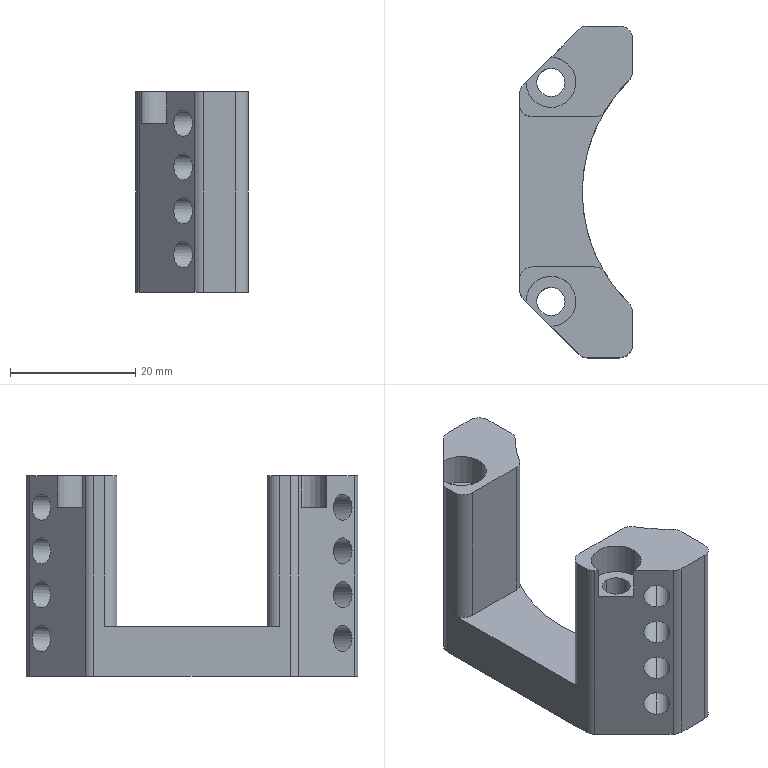CAM job | Mastercam | 3-axis milling, drilling | stock box 25 x 60 x 32 mm
Tools:
tool_number,name,type,diameter_mm,corner_radius_mm,flutes,flute_length_mm,overall_length_mm,shoulder_length_mm,holder_diameter_mm,length_offset,diameter_offset,default_rpm,default_feed_mm_min,default_plunge_mm_min,coolant
4,4 Flat End Mill,end mill,4,0,4,25,75,25,50,4,4,2500,300,600,COOL_OFF
5,4 Chamfer Mill,chamfer mill,4,0,4,25,75,30,50,5,5,6250,750,600,COOL_OFF
11,12 Flat End Mill,end mill,12,0,4,25,75,25,50,11,11,833,99.96,600,COOL_OFF
12,12 Flat End Mill,end mill,12,0,4,25,75,25,50,12,12,833,99.96,600,COOL_OFF
24,100 Flat End Mill,end mill,100,0,4,25,75,25,50,24,24,100,12,600,COOL_OFF
Operations:
seq,operation,operation_type,tool_number,tool_name,tool_diameter_mm,spindle_rpm,feed_mm_min,plunge_mm_min,retract_mm_min,cycle_time_s,wcs,posted,nc_file
1,Facing - [WCS: Plane] - [Tplane: Plane],Facing,24,100 Flat End Mill,100,4000,3000,600,1200,37.654,Plane,yes,.nc
2,3D High Speed (Dynamic OptiRough) - [WCS: Plane] - [Tplane: Plane],HighSpeed3D,11,12 Flat End Mill,12,7000,3000,600,1200,112.101,Plane,yes,.nc
3,Contour (Ramp) - [WCS: Plane] - [Tplane: Plane],Contour,4,4 Flat End Mill,4,6500,2500,600,1200,11.483,Plane,yes,.nc
4,Contour (2D) - [WCS: Plane] - [Tplane: Plane],Contour,4,4 Flat End Mill,4,6500,1000,600,1200,3.961,Plane,yes,.nc
5,2D High Speed (2D Area Mill) - [WCS: Plane] - [Tplane: Plane],HighSpeed2D,12,12 Flat End Mill,12,6000,1000,600,1200,8.271,Plane,yes,.nc
6,Contour (2D) - [WCS: Plane] - [Tplane: Plane],Contour,12,12 Flat End Mill,12,6000,1000,600,1200,29.607,Plane,yes,.nc
7,Contour (2D) - [WCS: Plane] - [Tplane: Plane],Contour,12,12 Flat End Mill,12,6000,1000,600,1200,11.519,Plane,yes,.nc
8,Drill/Counterbore - [WCS: Plane] - [Tplane: Plane],Drill,5,4 Chamfer Mill,4,6000,200,600,1200,1.977,Plane,yes,.nc
9,Contour (2D chamfer) - [WCS: Plane] - [Tplane: Plane],Contour,5,4 Chamfer Mill,4,6000,1000,600,1200,10.077,Plane,yes,.nc
10,2D High Speed (2D Area Mill) - [WCS: Plane-1] - [Tplane: Plane-1],HighSpeed2D,4,4 Flat End Mill,4,7000,3000,600,1200,189.428,Plane-1,yes,.nc
11,Contour (2D) - [WCS: Plane-1] - [Tplane: Plane-1],Contour,4,4 Flat End Mill,4,6000,1000,600,1200,8.694,Plane-1,yes,.nc
12,Contour (2D chamfer) - [WCS: Plane-1] - [Tplane: Plane-1],Contour,5,4 Chamfer Mill,4,6000,1000,600,1200,8.514,Plane-1,yes,.nc
13,Facing - [WCS: Plane-1] - [Tplane: Plane-1],Facing,24,100 Flat End Mill,100,4000,2000,600,1200,111.622,Plane-1,yes,.nc
14,Contour (2D chamfer) - [WCS: Plane-1] - [Tplane: Plane-1],Contour,5,4 Chamfer Mill,4,6000,1000,600,1200,9.004,Plane-1,yes,.nc
15,Drill/Counterbore - [WCS: Plane-2] - [Tplane: Plane-2],Drill,5,4 Chamfer Mill,4,6000,200,600,1200,3.758,Plane-2,yes,.nc
16,Drill/Counterbore - [WCS: Plane-3] - [Tplane: Plane-3],Drill,5,4 Chamfer Mill,4,6000,200,600,1200,3.758,Plane-3,yes,.nc